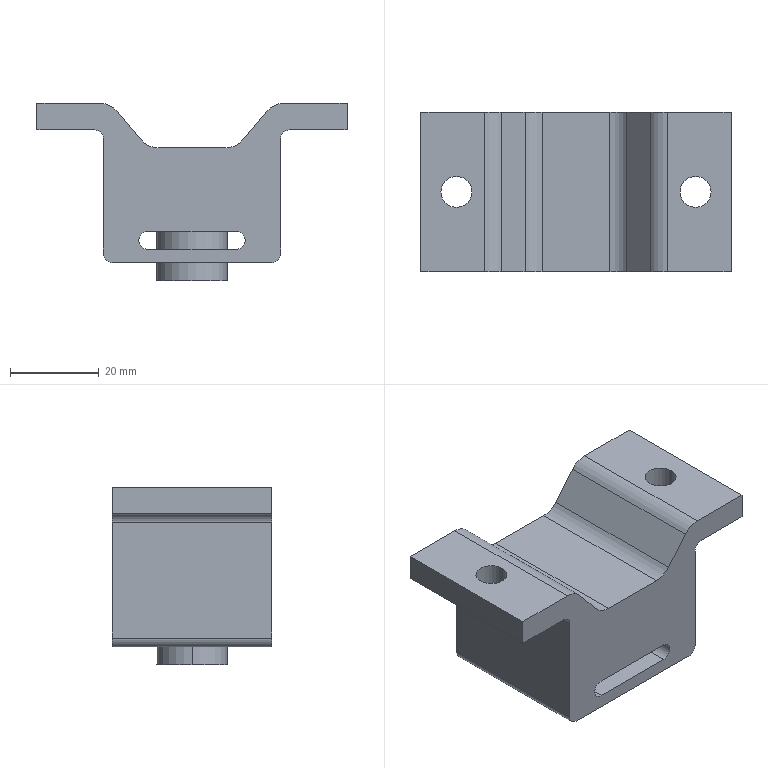Part | SolidWorks | features Fillet 3, ICE 3, Extrusion 1, HoleWzd 1 | 1 solid | 40 faces | box 70 x 36 x 40.002 mm | volume 44732 mm3 | cylinder 20 | plane 18 | cone 2 | commonest cylinder face diameters 4 x6 7 x4 10 x4 6.8 x2 16 x2 20 x2
STEP:
#1=CARTESIAN_POINT('',(3.4,18.,1.993));
#2=VERTEX_POINT('',#1);
#3=CARTESIAN_POINT('',(-3.4,18.,1.993));
#4=VERTEX_POINT('',#3);
#5=CARTESIAN_POINT('',(0.,18.,1.993));
#6=DIRECTION('',(0.,0.,-1.));
#7=DIRECTION('',(-1.,0.,0.));
#8=AXIS2_PLACEMENT_3D('',#5,#6,#7);
#9=CIRCLE('',#8,3.4);
#10=EDGE_CURVE('',#2,#4,#9,.T.);
#11=ORIENTED_EDGE('',*,*,#10,.F.);
#12=CARTESIAN_POINT('',(3.4,18.,-20.257));
#13=VERTEX_POINT('',#12);
#14=CARTESIAN_POINT('',(3.4,18.,-20.257));
#15=DIRECTION('',(0.,0.,-1.));
#16=VECTOR('',#15,1000.);
#17=LINE('',#14,#16);
#18=EDGE_CURVE('',#2,#13,#17,.T.);
#19=ORIENTED_EDGE('',*,*,#18,.T.);
#20=CARTESIAN_POINT('',(-3.4,18.,-20.257));
#21=VERTEX_POINT('',#20);
#22=CARTESIAN_POINT('',(0.,18.,-20.257));
#23=DIRECTION('',(0.,0.,-1.));
#24=DIRECTION('',(-1.,0.,0.));
#25=AXIS2_PLACEMENT_3D('',#22,#23,#24);
#26=CIRCLE('',#25,3.4);
#27=EDGE_CURVE('',#13,#21,#26,.T.);
#28=ORIENTED_EDGE('',*,*,#27,.T.);
#29=CARTESIAN_POINT('',(-3.4,18.,-20.257));
#30=DIRECTION('',(0.,0.,-1.));
#31=VECTOR('',#30,1000.);
#32=LINE('',#29,#31);
#33=EDGE_CURVE('',#4,#21,#32,.T.);
#34=ORIENTED_EDGE('',*,*,#33,.F.);
#35=EDGE_LOOP('',(#11,#19,#28,#34));
#36=FACE_OUTER_BOUND('',#35,.T.);
#37=CARTESIAN_POINT('',(0.,18.,-20.257));
#38=DIRECTION('',(0.,0.,-1.));
#39=DIRECTION('',(-1.,0.,0.));
#40=AXIS2_PLACEMENT_3D('',#37,#38,#39);
#41=CYLINDRICAL_SURFACE('',#40,3.4);
#42=ADVANCED_FACE('',(#36),#41,.F.);
#43=CARTESIAN_POINT('',(0.,18.,4.035));
#44=VERTEX_POINT('',#43);
#45=CARTESIAN_POINT('',(-3.4,18.,1.993));
#46=DIRECTION('',(-0.8572,0.,-0.515));
#47=VECTOR('',#46,1000.);
#48=LINE('',#45,#47);
#49=EDGE_CURVE('',#44,#4,#48,.T.);
#50=ORIENTED_EDGE('',*,*,#49,.F.);
#51=CARTESIAN_POINT('',(3.4,18.,1.993));
#52=DIRECTION('',(0.8572,0.,-0.515));
#53=VECTOR('',#52,1000.);
#54=LINE('',#51,#53);
#55=EDGE_CURVE('',#44,#2,#54,.T.);
#56=ORIENTED_EDGE('',*,*,#55,.T.);
#57=ORIENTED_EDGE('',*,*,#10,.T.);
#58=EDGE_LOOP('',(#50,#56,#57));
#59=FACE_OUTER_BOUND('',#58,.T.);
#60=CARTESIAN_POINT('',(0.,18.,1.993));
#61=DIRECTION('',(0.,0.,-1.));
#62=DIRECTION('',(-1.,0.,0.));
#63=AXIS2_PLACEMENT_3D('',#60,#61,#62);
#64=CONICAL_SURFACE('',#63,3.4,1.03);
#65=ADVANCED_FACE('',(#59),#64,.F.);
#66=CARTESIAN_POINT('',(-8.,18.,-20.257));
#67=VERTEX_POINT('',#66);
#68=CARTESIAN_POINT('',(8.,18.,-20.257));
#69=VERTEX_POINT('',#68);
#70=CARTESIAN_POINT('',(0.,18.,-20.257));
#71=DIRECTION('',(0.,0.,-1.));
#72=DIRECTION('',(-1.,0.,0.));
#73=AXIS2_PLACEMENT_3D('',#70,#71,#72);
#74=CIRCLE('',#73,8.);
#75=EDGE_CURVE('',#67,#69,#74,.T.);
#76=ORIENTED_EDGE('',*,*,#75,.F.);
#77=CARTESIAN_POINT('',(-8.,18.,-9.167));
#78=VERTEX_POINT('',#77);
#79=CARTESIAN_POINT('',(-8.,18.,-20.257));
#80=DIRECTION('',(0.,0.,1.));
#81=VECTOR('',#80,1000.);
#82=LINE('',#79,#81);
#83=EDGE_CURVE('',#67,#78,#82,.T.);
#84=ORIENTED_EDGE('',*,*,#83,.T.);
#85=CARTESIAN_POINT('',(8.,18.,-9.167));
#86=VERTEX_POINT('',#85);
#87=CARTESIAN_POINT('',(0.,18.,-9.167));
#88=DIRECTION('',(0.,0.,-1.));
#89=DIRECTION('',(-1.,0.,0.));
#90=AXIS2_PLACEMENT_3D('',#87,#88,#89);
#91=CIRCLE('',#90,8.);
#92=EDGE_CURVE('',#78,#86,#91,.T.);
#93=ORIENTED_EDGE('',*,*,#92,.T.);
#94=CARTESIAN_POINT('',(8.,18.,-20.257));
#95=DIRECTION('',(0.,0.,1.));
#96=VECTOR('',#95,1000.);
#97=LINE('',#94,#96);
#98=EDGE_CURVE('',#69,#86,#97,.T.);
#99=ORIENTED_EDGE('',*,*,#98,.F.);
#100=EDGE_LOOP('',(#76,#84,#93,#99));
#101=FACE_OUTER_BOUND('',#100,.T.);
#102=CARTESIAN_POINT('',(0.,18.,-20.257));
#103=DIRECTION('',(0.,0.,1.));
#104=DIRECTION('',(1.,0.,0.));
#105=AXIS2_PLACEMENT_3D('',#102,#103,#104);
#106=CYLINDRICAL_SURFACE('',#105,8.);
#107=ADVANCED_FACE('',(#101),#106,.T.);
#108=CARTESIAN_POINT('',(-10.,18.,-13.167));
#109=VERTEX_POINT('',#108);
#110=CARTESIAN_POINT('',(10.,18.,-13.167));
#111=VERTEX_POINT('',#110);
#112=CARTESIAN_POINT('',(0.,18.,-13.167));
#113=DIRECTION('',(0.,0.,1.));
#114=DIRECTION('',(1.,0.,0.));
#115=AXIS2_PLACEMENT_3D('',#112,#113,#114);
#116=CIRCLE('',#115,10.);
#117=EDGE_CURVE('',#109,#111,#116,.T.);
#118=ORIENTED_EDGE('',*,*,#117,.T.);
#119=CARTESIAN_POINT('',(10.,18.,-16.255));
#120=VERTEX_POINT('',#119);
#121=CARTESIAN_POINT('',(10.,18.,-10.255));
#122=DIRECTION('',(0.,0.,-1.));
#123=VECTOR('',#122,1000.);
#124=LINE('',#121,#123);
#125=EDGE_CURVE('',#111,#120,#124,.T.);
#126=ORIENTED_EDGE('',*,*,#125,.T.);
#127=CARTESIAN_POINT('',(-10.,18.,-16.255));
#128=VERTEX_POINT('',#127);
#129=CARTESIAN_POINT('',(0.,18.,-16.255));
#130=DIRECTION('',(0.,0.,-1.));
#131=DIRECTION('',(-1.,0.,0.));
#132=AXIS2_PLACEMENT_3D('',#129,#130,#131);
#133=CIRCLE('',#132,10.);
#134=EDGE_CURVE('',#120,#128,#133,.T.);
#135=ORIENTED_EDGE('',*,*,#134,.T.);
#136=CARTESIAN_POINT('',(-10.,18.,-10.255));
#137=DIRECTION('',(0.,0.,-1.));
#138=VECTOR('',#137,1000.);
#139=LINE('',#136,#138);
#140=EDGE_CURVE('',#109,#128,#139,.T.);
#141=ORIENTED_EDGE('',*,*,#140,.F.);
#142=EDGE_LOOP('',(#118,#126,#135,#141));
#143=FACE_OUTER_BOUND('',#142,.T.);
#144=CARTESIAN_POINT('',(0.,18.,-10.255));
#145=DIRECTION('',(0.,0.,-1.));
#146=DIRECTION('',(-1.,0.,0.));
#147=AXIS2_PLACEMENT_3D('',#144,#145,#146);
#148=CYLINDRICAL_SURFACE('',#147,10.);
#149=ADVANCED_FACE('',(#143),#148,.F.);
#150=CARTESIAN_POINT('',(-23.5,18.,19.745));
#151=VERTEX_POINT('',#150);
#152=CARTESIAN_POINT('',(-30.5,18.,19.745));
#153=VERTEX_POINT('',#152);
#154=CARTESIAN_POINT('',(-27.,18.,19.745));
#155=DIRECTION('',(0.,0.,-1.));
#156=DIRECTION('',(-1.,0.,0.));
#157=AXIS2_PLACEMENT_3D('',#154,#155,#156);
#158=CIRCLE('',#157,3.5);
#159=EDGE_CURVE('',#151,#153,#158,.T.);
#160=ORIENTED_EDGE('',*,*,#159,.F.);
#161=CARTESIAN_POINT('',(-23.5,18.,13.745));
#162=VERTEX_POINT('',#161);
#163=CARTESIAN_POINT('',(-23.5,18.,19.745));
#164=DIRECTION('',(0.,0.,-1.));
#165=VECTOR('',#164,1000.);
#166=LINE('',#163,#165);
#167=EDGE_CURVE('',#151,#162,#166,.T.);
#168=ORIENTED_EDGE('',*,*,#167,.T.);
#169=CARTESIAN_POINT('',(-30.5,18.,13.745));
#170=VERTEX_POINT('',#169);
#171=CARTESIAN_POINT('',(-27.,18.,13.745));
#172=DIRECTION('',(0.,0.,-1.));
#173=DIRECTION('',(-1.,0.,0.));
#174=AXIS2_PLACEMENT_3D('',#171,#172,#173);
#175=CIRCLE('',#174,3.5);
#176=EDGE_CURVE('',#162,#170,#175,.T.);
#177=ORIENTED_EDGE('',*,*,#176,.T.);
#178=CARTESIAN_POINT('',(-30.5,18.,19.745));
#179=DIRECTION('',(0.,0.,-1.));
#180=VECTOR('',#179,1000.);
#181=LINE('',#178,#180);
#182=EDGE_CURVE('',#153,#170,#181,.T.);
#183=ORIENTED_EDGE('',*,*,#182,.F.);
#184=EDGE_LOOP('',(#160,#168,#177,#183));
#185=FACE_OUTER_BOUND('',#184,.T.);
#186=CARTESIAN_POINT('',(-27.,18.,19.745));
#187=DIRECTION('',(0.,0.,-1.));
#188=DIRECTION('',(-1.,0.,0.));
#189=AXIS2_PLACEMENT_3D('',#186,#187,#188);
#190=CYLINDRICAL_SURFACE('',#189,3.5);
#191=ADVANCED_FACE('',(#185),#190,.F.);
#192=CARTESIAN_POINT('',(30.5,18.,19.745));
#193=VERTEX_POINT('',#192);
#194=CARTESIAN_POINT('',(23.5,18.,19.745));
#195=VERTEX_POINT('',#194);
#196=CARTESIAN_POINT('',(27.,18.,19.745));
#197=DIRECTION('',(0.,0.,-1.));
#198=DIRECTION('',(-1.,0.,0.));
#199=AXIS2_PLACEMENT_3D('',#196,#197,#198);
#200=CIRCLE('',#199,3.5);
#201=EDGE_CURVE('',#193,#195,#200,.T.);
#202=ORIENTED_EDGE('',*,*,#201,.F.);
#203=CARTESIAN_POINT('',(30.5,18.,13.745));
#204=VERTEX_POINT('',#203);
#205=CARTESIAN_POINT('',(30.5,18.,19.745));
#206=DIRECTION('',(0.,0.,-1.));
#207=VECTOR('',#206,1000.);
#208=LINE('',#205,#207);
#209=EDGE_CURVE('',#193,#204,#208,.T.);
#210=ORIENTED_EDGE('',*,*,#209,.T.);
#211=CARTESIAN_POINT('',(23.5,18.,13.745));
#212=VERTEX_POINT('',#211);
#213=CARTESIAN_POINT('',(27.,18.,13.745));
#214=DIRECTION('',(0.,0.,-1.));
#215=DIRECTION('',(-1.,0.,0.));
#216=AXIS2_PLACEMENT_3D('',#213,#214,#215);
#217=CIRCLE('',#216,3.5);
#218=EDGE_CURVE('',#204,#212,#217,.T.);
#219=ORIENTED_EDGE('',*,*,#218,.T.);
#220=CARTESIAN_POINT('',(23.5,18.,19.745));
#221=DIRECTION('',(0.,0.,-1.));
#222=VECTOR('',#221,1000.);
#223=LINE('',#220,#222);
#224=EDGE_CURVE('',#195,#212,#223,.T.);
#225=ORIENTED_EDGE('',*,*,#224,.F.);
#226=EDGE_LOOP('',(#202,#210,#219,#225));
#227=FACE_OUTER_BOUND('',#226,.T.);
#228=CARTESIAN_POINT('',(27.,18.,19.745));
#229=DIRECTION('',(0.,0.,-1.));
#230=DIRECTION('',(-1.,0.,0.));
#231=AXIS2_PLACEMENT_3D('',#228,#229,#230);
#232=CYLINDRICAL_SURFACE('',#231,3.5);
#233=ADVANCED_FACE('',(#227),#232,.F.);
#234=CARTESIAN_POINT('',(0.,18.,-13.167));
#235=DIRECTION('',(0.,0.,1.));
#236=DIRECTION('',(1.,0.,0.));
#237=AXIS2_PLACEMENT_3D('',#234,#235,#236);
#238=CIRCLE('',#237,10.);
#239=EDGE_CURVE('',#111,#109,#238,.T.);
#240=ORIENTED_EDGE('',*,*,#239,.F.);
#241=CARTESIAN_POINT('',(10.,36.,-13.167));
#242=VERTEX_POINT('',#241);
#243=CARTESIAN_POINT('',(10.,36.,-13.167));
#244=DIRECTION('',(0.,-1.,0.));
#245=VECTOR('',#244,1000.);
#246=LINE('',#243,#245);
#247=EDGE_CURVE('',#242,#111,#246,.T.);
#248=ORIENTED_EDGE('',*,*,#247,.F.);
#249=CARTESIAN_POINT('',(-10.,36.,-13.167));
#250=VERTEX_POINT('',#249);
#251=CARTESIAN_POINT('',(-10.,36.,-13.167));
#252=DIRECTION('',(-1.,0.,0.));
#253=VECTOR('',#252,1000.);
#254=LINE('',#251,#253);
#255=EDGE_CURVE('',#242,#250,#254,.T.);
#256=ORIENTED_EDGE('',*,*,#255,.T.);
#257=CARTESIAN_POINT('',(-10.,36.,-13.167));
#258=DIRECTION('',(0.,-1.,0.));
#259=VECTOR('',#258,1000.);
#260=LINE('',#257,#259);
#261=EDGE_CURVE('',#250,#109,#260,.T.);
#262=ORIENTED_EDGE('',*,*,#261,.T.);
#263=EDGE_LOOP('',(#240,#248,#256,#262));
#264=FACE_OUTER_BOUND('',#263,.T.);
#265=CARTESIAN_POINT('',(-10.,36.,-13.167));
#266=DIRECTION('',(0.,0.,1.));
#267=DIRECTION('',(1.,0.,0.));
#268=AXIS2_PLACEMENT_3D('',#265,#266,#267);
#269=PLANE('',#268);
#270=ADVANCED_FACE('',(#264),#269,.T.);
#271=CARTESIAN_POINT('',(18.,36.,-16.255));
#272=VERTEX_POINT('',#271);
#273=CARTESIAN_POINT('',(-18.,36.,-16.255));
#274=VERTEX_POINT('',#273);
#275=CARTESIAN_POINT('',(-20.,36.,-16.255));
#276=DIRECTION('',(-1.,0.,0.));
#277=VECTOR('',#276,1000.);
#278=LINE('',#275,#277);
#279=EDGE_CURVE('',#272,#274,#278,.T.);
#280=ORIENTED_EDGE('',*,*,#279,.T.);
#281=CARTESIAN_POINT('',(-20.,36.,-14.255));
#282=VERTEX_POINT('',#281);
#283=CARTESIAN_POINT('',(-18.,36.,-14.255));
#284=DIRECTION('',(0.,1.,0.));
#285=DIRECTION('',(0.,0.,-1.));
#286=AXIS2_PLACEMENT_3D('',#283,#284,#285);
#287=CIRCLE('',#286,2.);
#288=EDGE_CURVE('',#274,#282,#287,.T.);
#289=ORIENTED_EDGE('',*,*,#288,.T.);
#290=CARTESIAN_POINT('',(-20.,36.,11.745));
#291=VERTEX_POINT('',#290);
#292=CARTESIAN_POINT('',(-20.,36.,13.745));
#293=DIRECTION('',(0.,0.,1.));
#294=VECTOR('',#293,1000.);
#295=LINE('',#292,#294);
#296=EDGE_CURVE('',#282,#291,#295,.T.);
#297=ORIENTED_EDGE('',*,*,#296,.T.);
#298=CARTESIAN_POINT('',(-22.,36.,13.745));
#299=VERTEX_POINT('',#298);
#300=CARTESIAN_POINT('',(-22.,36.,11.745));
#301=DIRECTION('',(0.,-1.,0.));
#302=DIRECTION('',(0.,0.,-1.));
#303=AXIS2_PLACEMENT_3D('',#300,#301,#302);
#304=CIRCLE('',#303,2.);
#305=EDGE_CURVE('',#291,#299,#304,.T.);
#306=ORIENTED_EDGE('',*,*,#305,.T.);
#307=CARTESIAN_POINT('',(-35.,36.,13.745));
#308=VERTEX_POINT('',#307);
#309=CARTESIAN_POINT('',(-35.,36.,13.745));
#310=DIRECTION('',(-1.,0.,0.));
#311=VECTOR('',#310,1000.);
#312=LINE('',#309,#311);
#313=EDGE_CURVE('',#299,#308,#312,.T.);
#314=ORIENTED_EDGE('',*,*,#313,.T.);
#315=CARTESIAN_POINT('',(-35.,36.,19.745));
#316=VERTEX_POINT('',#315);
#317=CARTESIAN_POINT('',(-35.,36.,19.745));
#318=DIRECTION('',(0.,0.,1.));
#319=VECTOR('',#318,1000.);
#320=LINE('',#317,#319);
#321=EDGE_CURVE('',#308,#316,#320,.T.);
#322=ORIENTED_EDGE('',*,*,#321,.T.);
#323=CARTESIAN_POINT('',(-20.723,36.,19.745));
#324=VERTEX_POINT('',#323);
#325=CARTESIAN_POINT('',(-35.,36.,19.745));
#326=DIRECTION('',(1.,0.,0.));
#327=VECTOR('',#326,1000.);
#328=LINE('',#325,#327);
#329=EDGE_CURVE('',#316,#324,#328,.T.);
#330=ORIENTED_EDGE('',*,*,#329,.T.);
#331=CARTESIAN_POINT('',(-16.892,36.,17.959));
#332=VERTEX_POINT('',#331);
#333=CARTESIAN_POINT('',(-20.723,36.,14.745));
#334=DIRECTION('',(0.,1.,0.));
#335=DIRECTION('',(0.,0.,-1.));
#336=AXIS2_PLACEMENT_3D('',#333,#334,#335);
#337=CIRCLE('',#336,5.);
#338=EDGE_CURVE('',#324,#332,#337,.T.);
#339=ORIENTED_EDGE('',*,*,#338,.T.);
#340=CARTESIAN_POINT('',(-11.499,36.,11.531));
#341=VERTEX_POINT('',#340);
#342=CARTESIAN_POINT('',(-18.391,36.,19.745));
#343=DIRECTION('',(0.6428,0.,-0.766));
#344=VECTOR('',#343,1000.);
#345=LINE('',#342,#344);
#346=EDGE_CURVE('',#332,#341,#345,.T.);
#347=ORIENTED_EDGE('',*,*,#346,.T.);
#348=CARTESIAN_POINT('',(-7.668,36.,9.745));
#349=VERTEX_POINT('',#348);
#350=CARTESIAN_POINT('',(-7.668,36.,14.745));
#351=DIRECTION('',(0.,-1.,0.));
#352=DIRECTION('',(0.,0.,-1.));
#353=AXIS2_PLACEMENT_3D('',#350,#351,#352);
#354=CIRCLE('',#353,5.);
#355=EDGE_CURVE('',#341,#349,#354,.T.);
#356=ORIENTED_EDGE('',*,*,#355,.T.);
#357=CARTESIAN_POINT('',(7.668,36.,9.745));
#358=VERTEX_POINT('',#357);
#359=CARTESIAN_POINT('',(-10.,36.,9.745));
#360=DIRECTION('',(1.,0.,0.));
#361=VECTOR('',#360,1000.);
#362=LINE('',#359,#361);
#363=EDGE_CURVE('',#349,#358,#362,.T.);
#364=ORIENTED_EDGE('',*,*,#363,.T.);
#365=CARTESIAN_POINT('',(11.499,36.,11.531));
#366=VERTEX_POINT('',#365);
#367=CARTESIAN_POINT('',(7.668,36.,14.745));
#368=DIRECTION('',(0.,-1.,0.));
#369=DIRECTION('',(0.,0.,-1.));
#370=AXIS2_PLACEMENT_3D('',#367,#368,#369);
#371=CIRCLE('',#370,5.);
#372=EDGE_CURVE('',#358,#366,#371,.T.);
#373=ORIENTED_EDGE('',*,*,#372,.T.);
#374=CARTESIAN_POINT('',(16.892,36.,17.959));
#375=VERTEX_POINT('',#374);
#376=CARTESIAN_POINT('',(10.,36.,9.745));
#377=DIRECTION('',(0.6428,0.,0.766));
#378=VECTOR('',#377,1000.);
#379=LINE('',#376,#378);
#380=EDGE_CURVE('',#366,#375,#379,.T.);
#381=ORIENTED_EDGE('',*,*,#380,.T.);
#382=CARTESIAN_POINT('',(20.723,36.,19.745));
#383=VERTEX_POINT('',#382);
#384=CARTESIAN_POINT('',(20.723,36.,14.745));
#385=DIRECTION('',(0.,1.,0.));
#386=DIRECTION('',(0.,0.,-1.));
#387=AXIS2_PLACEMENT_3D('',#384,#385,#386);
#388=CIRCLE('',#387,5.);
#389=EDGE_CURVE('',#375,#383,#388,.T.);
#390=ORIENTED_EDGE('',*,*,#389,.T.);
#391=CARTESIAN_POINT('',(35.,36.,19.745));
#392=VERTEX_POINT('',#391);
#393=CARTESIAN_POINT('',(18.391,36.,19.745));
#394=DIRECTION('',(1.,0.,0.));
#395=VECTOR('',#394,1000.);
#396=LINE('',#393,#395);
#397=EDGE_CURVE('',#383,#392,#396,.T.);
#398=ORIENTED_EDGE('',*,*,#397,.T.);
#399=CARTESIAN_POINT('',(35.,36.,13.745));
#400=VERTEX_POINT('',#399);
#401=CARTESIAN_POINT('',(35.,36.,19.745));
#402=DIRECTION('',(0.,0.,-1.));
#403=VECTOR('',#402,1000.);
#404=LINE('',#401,#403);
#405=EDGE_CURVE('',#392,#400,#404,.T.);
#406=ORIENTED_EDGE('',*,*,#405,.T.);
#407=CARTESIAN_POINT('',(22.,36.,13.745));
#408=VERTEX_POINT('',#407);
#409=CARTESIAN_POINT('',(20.,36.,13.745));
#410=DIRECTION('',(-1.,0.,0.));
#411=VECTOR('',#410,1000.);
#412=LINE('',#409,#411);
#413=EDGE_CURVE('',#400,#408,#412,.T.);
#414=ORIENTED_EDGE('',*,*,#413,.T.);
#415=CARTESIAN_POINT('',(20.,36.,11.745));
#416=VERTEX_POINT('',#415);
#417=CARTESIAN_POINT('',(22.,36.,11.745));
#418=DIRECTION('',(0.,-1.,0.));
#419=DIRECTION('',(0.,0.,-1.));
#420=AXIS2_PLACEMENT_3D('',#417,#418,#419);
#421=CIRCLE('',#420,2.);
#422=EDGE_CURVE('',#408,#416,#421,.T.);
#423=ORIENTED_EDGE('',*,*,#422,.T.);
#424=CARTESIAN_POINT('',(20.,36.,-14.255));
#425=VERTEX_POINT('',#424);
#426=CARTESIAN_POINT('',(20.,36.,13.745));
#427=DIRECTION('',(0.,0.,-1.));
#428=VECTOR('',#427,1000.);
#429=LINE('',#426,#428);
#430=EDGE_CURVE('',#416,#425,#429,.T.);
#431=ORIENTED_EDGE('',*,*,#430,.T.);
#432=CARTESIAN_POINT('',(18.,36.,-14.255));
#433=DIRECTION('',(0.,1.,0.));
#434=DIRECTION('',(0.,0.,-1.));
#435=AXIS2_PLACEMENT_3D('',#432,#433,#434);
#436=CIRCLE('',#435,2.);
#437=EDGE_CURVE('',#425,#272,#436,.T.);
#438=ORIENTED_EDGE('',*,*,#437,.T.);
#439=EDGE_LOOP('',(#280,#289,#297,#306,#314,#322,#330,#339,#347,#356,#364,#373,#381,#390,#398,#406,#414,#423,#431,#438));
#440=FACE_OUTER_BOUND('',#439,.T.);
#441=CARTESIAN_POINT('',(-10.,36.,-9.167));
#442=VERTEX_POINT('',#441);
#443=CARTESIAN_POINT('',(-10.,36.,-11.167));
#444=DIRECTION('',(0.,1.,0.));
#445=DIRECTION('',(0.,0.,1.));
#446=AXIS2_PLACEMENT_3D('',#443,#444,#445);
#447=CIRCLE('',#446,2.);
#448=EDGE_CURVE('',#250,#442,#447,.T.);
#449=ORIENTED_EDGE('',*,*,#448,.F.);
#450=ORIENTED_EDGE('',*,*,#255,.F.);
#451=CARTESIAN_POINT('',(10.,36.,-9.167));
#452=VERTEX_POINT('',#451);
#453=CARTESIAN_POINT('',(10.,36.,-11.167));
#454=DIRECTION('',(0.,1.,0.));
#455=DIRECTION('',(0.,0.,1.));
#456=AXIS2_PLACEMENT_3D('',#453,#454,#455);
#457=CIRCLE('',#456,2.);
#458=EDGE_CURVE('',#452,#242,#457,.T.);
#459=ORIENTED_EDGE('',*,*,#458,.F.);
#460=CARTESIAN_POINT('',(-10.,36.,-9.167));
#461=DIRECTION('',(1.,0.,0.));
#462=VECTOR('',#461,1000.);
#463=LINE('',#460,#462);
#464=EDGE_CURVE('',#442,#452,#463,.T.);
#465=ORIENTED_EDGE('',*,*,#464,.F.);
#466=EDGE_LOOP('',(#449,#450,#459,#465));
#467=FACE_BOUND('',#466,.T.);
#468=CARTESIAN_POINT('',(0.,36.,0.));
#469=DIRECTION('',(0.,-1.,0.));
#470=DIRECTION('',(0.,0.,-1.));
#471=AXIS2_PLACEMENT_3D('',#468,#469,#470);
#472=PLANE('',#471);
#473=ADVANCED_FACE('',(#440,#467),#472,.F.);
#474=CARTESIAN_POINT('',(-20.,0.,-14.255));
#475=VERTEX_POINT('',#474);
#476=CARTESIAN_POINT('',(-20.,0.,11.745));
#477=VERTEX_POINT('',#476);
#478=CARTESIAN_POINT('',(-20.,0.,13.745));
#479=DIRECTION('',(0.,0.,1.));
#480=VECTOR('',#479,1000.);
#481=LINE('',#478,#480);
#482=EDGE_CURVE('',#475,#477,#481,.T.);
#483=ORIENTED_EDGE('',*,*,#482,.F.);
#484=CARTESIAN_POINT('',(-18.,0.,-16.255));
#485=VERTEX_POINT('',#484);
#486=CARTESIAN_POINT('',(-18.,0.,-14.255));
#487=DIRECTION('',(0.,-1.,0.));
#488=DIRECTION('',(0.,0.,-1.));
#489=AXIS2_PLACEMENT_3D('',#486,#487,#488);
#490=CIRCLE('',#489,2.);
#491=EDGE_CURVE('',#475,#485,#490,.T.);
#492=ORIENTED_EDGE('',*,*,#491,.T.);
#493=CARTESIAN_POINT('',(18.,0.,-16.255));
#494=VERTEX_POINT('',#493);
#495=CARTESIAN_POINT('',(-20.,0.,-16.255));
#496=DIRECTION('',(-1.,0.,0.));
#497=VECTOR('',#496,1000.);
#498=LINE('',#495,#497);
#499=EDGE_CURVE('',#494,#485,#498,.T.);
#500=ORIENTED_EDGE('',*,*,#499,.F.);
#501=CARTESIAN_POINT('',(20.,0.,-14.255));
#502=VERTEX_POINT('',#501);
#503=CARTESIAN_POINT('',(18.,0.,-14.255));
#504=DIRECTION('',(0.,-1.,0.));
#505=DIRECTION('',(0.,0.,-1.));
#506=AXIS2_PLACEMENT_3D('',#503,#504,#505);
#507=CIRCLE('',#506,2.);
#508=EDGE_CURVE('',#494,#502,#507,.T.);
#509=ORIENTED_EDGE('',*,*,#508,.T.);
#510=CARTESIAN_POINT('',(20.,0.,11.745));
#511=VERTEX_POINT('',#510);
#512=CARTESIAN_POINT('',(20.,0.,13.745));
#513=DIRECTION('',(0.,0.,-1.));
#514=VECTOR('',#513,1000.);
#515=LINE('',#512,#514);
#516=EDGE_CURVE('',#511,#502,#515,.T.);
#517=ORIENTED_EDGE('',*,*,#516,.F.);
#518=CARTESIAN_POINT('',(22.,0.,13.745));
#519=VERTEX_POINT('',#518);
#520=CARTESIAN_POINT('',(22.,0.,11.745));
#521=DIRECTION('',(0.,1.,0.));
#522=DIRECTION('',(0.,0.,-1.));
#523=AXIS2_PLACEMENT_3D('',#520,#521,#522);
#524=CIRCLE('',#523,2.);
#525=EDGE_CURVE('',#511,#519,#524,.T.);
#526=ORIENTED_EDGE('',*,*,#525,.T.);
#527=CARTESIAN_POINT('',(35.,0.,13.745));
#528=VERTEX_POINT('',#527);
#529=CARTESIAN_POINT('',(20.,0.,13.745));
#530=DIRECTION('',(-1.,0.,0.));
#531=VECTOR('',#530,1000.);
#532=LINE('',#529,#531);
#533=EDGE_CURVE('',#528,#519,#532,.T.);
#534=ORIENTED_EDGE('',*,*,#533,.F.);
#535=CARTESIAN_POINT('',(35.,0.,19.745));
#536=VERTEX_POINT('',#535);
#537=CARTESIAN_POINT('',(35.,0.,19.745));
#538=DIRECTION('',(0.,0.,-1.));
#539=VECTOR('',#538,1000.);
#540=LINE('',#537,#539);
#541=EDGE_CURVE('',#536,#528,#540,.T.);
#542=ORIENTED_EDGE('',*,*,#541,.F.);
#543=CARTESIAN_POINT('',(20.723,0.,19.745));
#544=VERTEX_POINT('',#543);
#545=CARTESIAN_POINT('',(18.391,0.,19.745));
#546=DIRECTION('',(1.,0.,0.));
#547=VECTOR('',#546,1000.);
#548=LINE('',#545,#547);
#549=EDGE_CURVE('',#544,#536,#548,.T.);
#550=ORIENTED_EDGE('',*,*,#549,.F.);
#551=CARTESIAN_POINT('',(16.892,0.,17.959));
#552=VERTEX_POINT('',#551);
#553=CARTESIAN_POINT('',(20.723,0.,14.745));
#554=DIRECTION('',(0.,-1.,0.));
#555=DIRECTION('',(0.,0.,-1.));
#556=AXIS2_PLACEMENT_3D('',#553,#554,#555);
#557=CIRCLE('',#556,5.);
#558=EDGE_CURVE('',#544,#552,#557,.T.);
#559=ORIENTED_EDGE('',*,*,#558,.T.);
#560=CARTESIAN_POINT('',(11.499,0.,11.531));
#561=VERTEX_POINT('',#560);
#562=CARTESIAN_POINT('',(10.,0.,9.745));
#563=DIRECTION('',(0.6428,0.,0.766));
#564=VECTOR('',#563,1000.);
#565=LINE('',#562,#564);
#566=EDGE_CURVE('',#561,#552,#565,.T.);
#567=ORIENTED_EDGE('',*,*,#566,.F.);
#568=CARTESIAN_POINT('',(7.668,0.,9.745));
#569=VERTEX_POINT('',#568);
#570=CARTESIAN_POINT('',(7.668,0.,14.745));
#571=DIRECTION('',(0.,1.,0.));
#572=DIRECTION('',(0.,0.,-1.));
#573=AXIS2_PLACEMENT_3D('',#570,#571,#572);
#574=CIRCLE('',#573,5.);
#575=EDGE_CURVE('',#561,#569,#574,.T.);
#576=ORIENTED_EDGE('',*,*,#575,.T.);
#577=CARTESIAN_POINT('',(-7.668,0.,9.745));
#578=VERTEX_POINT('',#577);
#579=CARTESIAN_POINT('',(-10.,0.,9.745));
#580=DIRECTION('',(1.,0.,0.));
#581=VECTOR('',#580,1000.);
#582=LINE('',#579,#581);
#583=EDGE_CURVE('',#578,#569,#582,.T.);
#584=ORIENTED_EDGE('',*,*,#583,.F.);
#585=CARTESIAN_POINT('',(-11.499,0.,11.531));
#586=VERTEX_POINT('',#585);
#587=CARTESIAN_POINT('',(-7.668,0.,14.745));
#588=DIRECTION('',(0.,1.,0.));
#589=DIRECTION('',(0.,0.,-1.));
#590=AXIS2_PLACEMENT_3D('',#587,#588,#589);
#591=CIRCLE('',#590,5.);
#592=EDGE_CURVE('',#578,#586,#591,.T.);
#593=ORIENTED_EDGE('',*,*,#592,.T.);
#594=CARTESIAN_POINT('',(-16.892,0.,17.959));
#595=VERTEX_POINT('',#594);
#596=CARTESIAN_POINT('',(-18.391,0.,19.745));
#597=DIRECTION('',(0.6428,0.,-0.766));
#598=VECTOR('',#597,1000.);
#599=LINE('',#596,#598);
#600=EDGE_CURVE('',#595,#586,#599,.T.);
#601=ORIENTED_EDGE('',*,*,#600,.F.);
#602=CARTESIAN_POINT('',(-20.723,0.,19.745));
#603=VERTEX_POINT('',#602);
#604=CARTESIAN_POINT('',(-20.723,0.,14.745));
#605=DIRECTION('',(0.,-1.,0.));
#606=DIRECTION('',(0.,0.,-1.));
#607=AXIS2_PLACEMENT_3D('',#604,#605,#606);
#608=CIRCLE('',#607,5.);
#609=EDGE_CURVE('',#595,#603,#608,.T.);
#610=ORIENTED_EDGE('',*,*,#609,.T.);
#611=CARTESIAN_POINT('',(-35.,0.,19.745));
#612=VERTEX_POINT('',#611);
#613=CARTESIAN_POINT('',(-35.,0.,19.745));
#614=DIRECTION('',(1.,0.,0.));
#615=VECTOR('',#614,1000.);
#616=LINE('',#613,#615);
#617=EDGE_CURVE('',#612,#603,#616,.T.);
#618=ORIENTED_EDGE('',*,*,#617,.F.);
#619=CARTESIAN_POINT('',(-35.,0.,13.745));
#620=VERTEX_POINT('',#619);
#621=CARTESIAN_POINT('',(-35.,0.,19.745));
#622=DIRECTION('',(0.,0.,1.));
#623=VECTOR('',#622,1000.);
#624=LINE('',#621,#623);
#625=EDGE_CURVE('',#620,#612,#624,.T.);
#626=ORIENTED_EDGE('',*,*,#625,.F.);
#627=CARTESIAN_POINT('',(-22.,0.,13.745));
#628=VERTEX_POINT('',#627);
#629=CARTESIAN_POINT('',(-35.,0.,13.745));
#630=DIRECTION('',(-1.,0.,0.));
#631=VECTOR('',#630,1000.);
#632=LINE('',#629,#631);
#633=EDGE_CURVE('',#628,#620,#632,.T.);
#634=ORIENTED_EDGE('',*,*,#633,.F.);
#635=CARTESIAN_POINT('',(-22.,0.,11.745));
#636=DIRECTION('',(0.,1.,0.));
#637=DIRECTION('',(0.,0.,-1.));
#638=AXIS2_PLACEMENT_3D('',#635,#636,#637);
#639=CIRCLE('',#638,2.);
#640=EDGE_CURVE('',#628,#477,#639,.T.);
#641=ORIENTED_EDGE('',*,*,#640,.T.);
#642=EDGE_LOOP('',(#483,#492,#500,#509,#517,#526,#534,#542,#550,#559,#567,#576,#584,#593,#601,#610,#618,#626,#634,#641));
#643=FACE_OUTER_BOUND('',#642,.T.);
#644=CARTESIAN_POINT('',(10.,0.,-13.167));
#645=VERTEX_POINT('',#644);
#646=CARTESIAN_POINT('',(-10.,0.,-13.167));
#647=VERTEX_POINT('',#646);
#648=CARTESIAN_POINT('',(-10.,0.,-13.167));
#649=DIRECTION('',(-1.,0.,0.));
#650=VECTOR('',#649,1000.);
#651=LINE('',#648,#650);
#652=EDGE_CURVE('',#645,#647,#651,.T.);
#653=ORIENTED_EDGE('',*,*,#652,.T.);
#654=CARTESIAN_POINT('',(-10.,0.,-9.167));
#655=VERTEX_POINT('',#654);
#656=CARTESIAN_POINT('',(-10.,0.,-11.167));
#657=DIRECTION('',(0.,1.,0.));
#658=DIRECTION('',(0.,0.,1.));
#659=AXIS2_PLACEMENT_3D('',#656,#657,#658);
#660=CIRCLE('',#659,2.);
#661=EDGE_CURVE('',#647,#655,#660,.T.);
#662=ORIENTED_EDGE('',*,*,#661,.T.);
#663=CARTESIAN_POINT('',(10.,0.,-9.167));
#664=VERTEX_POINT('',#663);
#665=CARTESIAN_POINT('',(-10.,0.,-9.167));
#666=DIRECTION('',(1.,0.,0.));
#667=VECTOR('',#666,1000.);
#668=LINE('',#665,#667);
#669=EDGE_CURVE('',#655,#664,#668,.T.);
#670=ORIENTED_EDGE('',*,*,#669,.T.);
#671=CARTESIAN_POINT('',(10.,0.,-11.167));
#672=DIRECTION('',(0.,1.,0.));
#673=DIRECTION('',(0.,0.,1.));
#674=AXIS2_PLACEMENT_3D('',#671,#672,#673);
#675=CIRCLE('',#674,2.);
#676=EDGE_CURVE('',#664,#645,#675,.T.);
#677=ORIENTED_EDGE('',*,*,#676,.T.);
#678=EDGE_LOOP('',(#653,#662,#670,#677));
#679=FACE_BOUND('',#678,.T.);
#680=CARTESIAN_POINT('',(0.,0.,0.));
#681=DIRECTION('',(0.,-1.,0.));
#682=DIRECTION('',(0.,0.,-1.));
#683=AXIS2_PLACEMENT_3D('',#680,#681,#682);
#684=PLANE('',#683);
#685=ADVANCED_FACE('',(#643,#679),#684,.T.);
#686=ORIENTED_EDGE('',*,*,#516,.T.);
#687=CARTESIAN_POINT('',(20.,36.,-14.255));
#688=DIRECTION('',(0.,1.,0.));
#689=VECTOR('',#688,1000.);
#690=LINE('',#687,#689);
#691=EDGE_CURVE('',#502,#425,#690,.T.);
#692=ORIENTED_EDGE('',*,*,#691,.T.);
#693=ORIENTED_EDGE('',*,*,#430,.F.);
#694=CARTESIAN_POINT('',(20.,0.,11.745));
#695=DIRECTION('',(0.,-1.,0.));
#696=VECTOR('',#695,1000.);
#697=LINE('',#694,#696);
#698=EDGE_CURVE('',#416,#511,#697,.T.);
#699=ORIENTED_EDGE('',*,*,#698,.T.);
#700=EDGE_LOOP('',(#686,#692,#693,#699));
#701=FACE_OUTER_BOUND('',#700,.T.);
#702=CARTESIAN_POINT('',(20.,36.,13.745));
#703=DIRECTION('',(-1.,0.,0.));
#704=DIRECTION('',(0.,0.,1.));
#705=AXIS2_PLACEMENT_3D('',#702,#703,#704);
#706=PLANE('',#705);
#707=ADVANCED_FACE('',(#701),#706,.F.);
#708=CARTESIAN_POINT('',(0.,18.,-16.255));
#709=DIRECTION('',(0.,0.,-1.));
#710=DIRECTION('',(-1.,0.,0.));
#711=AXIS2_PLACEMENT_3D('',#708,#709,#710);
#712=CIRCLE('',#711,10.);
#713=EDGE_CURVE('',#128,#120,#712,.T.);
#714=ORIENTED_EDGE('',*,*,#713,.F.);
#715=ORIENTED_EDGE('',*,*,#134,.F.);
#716=EDGE_LOOP('',(#714,#715));
#717=FACE_BOUND('',#716,.T.);
#718=ORIENTED_EDGE('',*,*,#499,.T.);
#719=CARTESIAN_POINT('',(-18.,36.,-16.255));
#720=DIRECTION('',(0.,1.,0.));
#721=VECTOR('',#720,1000.);
#722=LINE('',#719,#721);
#723=EDGE_CURVE('',#485,#274,#722,.T.);
#724=ORIENTED_EDGE('',*,*,#723,.T.);
#725=ORIENTED_EDGE('',*,*,#279,.F.);
#726=CARTESIAN_POINT('',(18.,36.,-16.255));
#727=DIRECTION('',(0.,-1.,0.));
#728=VECTOR('',#727,1000.);
#729=LINE('',#726,#728);
#730=EDGE_CURVE('',#272,#494,#729,.T.);
#731=ORIENTED_EDGE('',*,*,#730,.T.);
#732=EDGE_LOOP('',(#718,#724,#725,#731));
#733=FACE_OUTER_BOUND('',#732,.T.);
#734=CARTESIAN_POINT('',(-20.,36.,-16.255));
#735=DIRECTION('',(0.,0.,1.));
#736=DIRECTION('',(1.,0.,0.));
#737=AXIS2_PLACEMENT_3D('',#734,#735,#736);
#738=PLANE('',#737);
#739=ADVANCED_FACE('',(#717,#733),#738,.F.);
#740=ORIENTED_EDGE('',*,*,#296,.F.);
#741=CARTESIAN_POINT('',(-20.,36.,-14.255));
#742=DIRECTION('',(0.,-1.,0.));
#743=VECTOR('',#742,1000.);
#744=LINE('',#741,#743);
#745=EDGE_CURVE('',#282,#475,#744,.T.);
#746=ORIENTED_EDGE('',*,*,#745,.T.);
#747=ORIENTED_EDGE('',*,*,#482,.T.);
#748=CARTESIAN_POINT('',(-20.,36.,11.745));
#749=DIRECTION('',(0.,1.,0.));
#750=VECTOR('',#749,1000.);
#751=LINE('',#748,#750);
#752=EDGE_CURVE('',#477,#291,#751,.T.);
#753=ORIENTED_EDGE('',*,*,#752,.T.);
#754=EDGE_LOOP('',(#740,#746,#747,#753));
#755=FACE_OUTER_BOUND('',#754,.T.);
#756=CARTESIAN_POINT('',(-20.,36.,13.745));
#757=DIRECTION('',(1.,0.,0.));
#758=DIRECTION('',(0.,0.,-1.));
#759=AXIS2_PLACEMENT_3D('',#756,#757,#758);
#760=PLANE('',#759);
#761=ADVANCED_FACE('',(#755),#760,.F.);
#762=CARTESIAN_POINT('',(-27.,18.,13.745));
#763=DIRECTION('',(0.,0.,-1.));
#764=DIRECTION('',(-1.,0.,0.));
#765=AXIS2_PLACEMENT_3D('',#762,#763,#764);
#766=CIRCLE('',#765,3.5);
#767=EDGE_CURVE('',#170,#162,#766,.T.);
#768=ORIENTED_EDGE('',*,*,#767,.F.);
#769=ORIENTED_EDGE('',*,*,#176,.F.);
#770=EDGE_LOOP('',(#768,#769));
#771=FACE_BOUND('',#770,.T.);
#772=ORIENTED_EDGE('',*,*,#313,.F.);
#773=CARTESIAN_POINT('',(-22.,0.,13.745));
#774=DIRECTION('',(0.,-1.,0.));
#775=VECTOR('',#774,1000.);
#776=LINE('',#773,#775);
#777=EDGE_CURVE('',#299,#628,#776,.T.);
#778=ORIENTED_EDGE('',*,*,#777,.T.);
#779=ORIENTED_EDGE('',*,*,#633,.T.);
#780=CARTESIAN_POINT('',(-35.,36.,13.745));
#781=DIRECTION('',(0.,-1.,0.));
#782=VECTOR('',#781,1000.);
#783=LINE('',#780,#782);
#784=EDGE_CURVE('',#308,#620,#783,.T.);
#785=ORIENTED_EDGE('',*,*,#784,.F.);
#786=EDGE_LOOP('',(#772,#778,#779,#785));
#787=FACE_OUTER_BOUND('',#786,.T.);
#788=CARTESIAN_POINT('',(-35.,36.,13.745));
#789=DIRECTION('',(0.,0.,1.));
#790=DIRECTION('',(1.,0.,0.));
#791=AXIS2_PLACEMENT_3D('',#788,#789,#790);
#792=PLANE('',#791);
#793=ADVANCED_FACE('',(#771,#787),#792,.F.);
#794=ORIENTED_EDGE('',*,*,#625,.T.);
#795=CARTESIAN_POINT('',(-35.,36.,19.745));
#796=DIRECTION('',(0.,-1.,0.));
#797=VECTOR('',#796,1000.);
#798=LINE('',#795,#797);
#799=EDGE_CURVE('',#316,#612,#798,.T.);
#800=ORIENTED_EDGE('',*,*,#799,.F.);
#801=ORIENTED_EDGE('',*,*,#321,.F.);
#802=ORIENTED_EDGE('',*,*,#784,.T.);
#803=EDGE_LOOP('',(#794,#800,#801,#802));
#804=FACE_OUTER_BOUND('',#803,.T.);
#805=CARTESIAN_POINT('',(-35.,36.,19.745));
#806=DIRECTION('',(1.,0.,0.));
#807=DIRECTION('',(0.,0.,-1.));
#808=AXIS2_PLACEMENT_3D('',#805,#806,#807);
#809=PLANE('',#808);
#810=ADVANCED_FACE('',(#804),#809,.F.);
#811=CARTESIAN_POINT('',(-27.,18.,19.745));
#812=DIRECTION('',(0.,0.,-1.));
#813=DIRECTION('',(-1.,0.,0.));
#814=AXIS2_PLACEMENT_3D('',#811,#812,#813);
#815=CIRCLE('',#814,3.5);
#816=EDGE_CURVE('',#153,#151,#815,.T.);
#817=ORIENTED_EDGE('',*,*,#816,.T.);
#818=ORIENTED_EDGE('',*,*,#159,.T.);
#819=EDGE_LOOP('',(#817,#818));
#820=FACE_BOUND('',#819,.T.);
#821=ORIENTED_EDGE('',*,*,#617,.T.);
#822=CARTESIAN_POINT('',(-20.723,36.,19.745));
#823=DIRECTION('',(0.,1.,0.));
#824=VECTOR('',#823,1000.);
#825=LINE('',#822,#824);
#826=EDGE_CURVE('',#603,#324,#825,.T.);
#827=ORIENTED_EDGE('',*,*,#826,.T.);
#828=ORIENTED_EDGE('',*,*,#329,.F.);
#829=ORIENTED_EDGE('',*,*,#799,.T.);
#830=EDGE_LOOP('',(#821,#827,#828,#829));
#831=FACE_OUTER_BOUND('',#830,.T.);
#832=CARTESIAN_POINT('',(-35.,36.,19.745));
#833=DIRECTION('',(0.,0.,-1.));
#834=DIRECTION('',(-1.,0.,0.));
#835=AXIS2_PLACEMENT_3D('',#832,#833,#834);
#836=PLANE('',#835);
#837=ADVANCED_FACE('',(#820,#831),#836,.F.);
#838=ORIENTED_EDGE('',*,*,#600,.T.);
#839=CARTESIAN_POINT('',(-11.499,36.,11.531));
#840=DIRECTION('',(0.,1.,0.));
#841=VECTOR('',#840,1000.);
#842=LINE('',#839,#841);
#843=EDGE_CURVE('',#586,#341,#842,.T.);
#844=ORIENTED_EDGE('',*,*,#843,.T.);
#845=ORIENTED_EDGE('',*,*,#346,.F.);
#846=CARTESIAN_POINT('',(-16.892,36.,17.959));
#847=DIRECTION('',(0.,-1.,0.));
#848=VECTOR('',#847,1000.);
#849=LINE('',#846,#848);
#850=EDGE_CURVE('',#332,#595,#849,.T.);
#851=ORIENTED_EDGE('',*,*,#850,.T.);
#852=EDGE_LOOP('',(#838,#844,#845,#851));
#853=FACE_OUTER_BOUND('',#852,.T.);
#854=CARTESIAN_POINT('',(-18.391,36.,19.745));
#855=DIRECTION('',(-0.766,0.,-0.6428));
#856=DIRECTION('',(-0.6428,0.,0.766));
#857=AXIS2_PLACEMENT_3D('',#854,#855,#856);
#858=PLANE('',#857);
#859=ADVANCED_FACE('',(#853),#858,.F.);
#860=ORIENTED_EDGE('',*,*,#583,.T.);
#861=CARTESIAN_POINT('',(7.668,36.,9.745));
#862=DIRECTION('',(0.,1.,0.));
#863=VECTOR('',#862,1000.);
#864=LINE('',#861,#863);
#865=EDGE_CURVE('',#569,#358,#864,.T.);
#866=ORIENTED_EDGE('',*,*,#865,.T.);
#867=ORIENTED_EDGE('',*,*,#363,.F.);
#868=CARTESIAN_POINT('',(-7.668,0.,9.745));
#869=DIRECTION('',(0.,-1.,0.));
#870=VECTOR('',#869,1000.);
#871=LINE('',#868,#870);
#872=EDGE_CURVE('',#349,#578,#871,.T.);
#873=ORIENTED_EDGE('',*,*,#872,.T.);
#874=EDGE_LOOP('',(#860,#866,#867,#873));
#875=FACE_OUTER_BOUND('',#874,.T.);
#876=CARTESIAN_POINT('',(-10.,36.,9.745));
#877=DIRECTION('',(0.,0.,-1.));
#878=DIRECTION('',(-1.,0.,0.));
#879=AXIS2_PLACEMENT_3D('',#876,#877,#878);
#880=PLANE('',#879);
#881=ADVANCED_FACE('',(#875),#880,.F.);
#882=ORIENTED_EDGE('',*,*,#566,.T.);
#883=CARTESIAN_POINT('',(16.892,36.,17.959));
#884=DIRECTION('',(0.,1.,0.));
#885=VECTOR('',#884,1000.);
#886=LINE('',#883,#885);
#887=EDGE_CURVE('',#552,#375,#886,.T.);
#888=ORIENTED_EDGE('',*,*,#887,.T.);
#889=ORIENTED_EDGE('',*,*,#380,.F.);
#890=CARTESIAN_POINT('',(11.499,0.,11.531));
#891=DIRECTION('',(0.,-1.,0.));
#892=VECTOR('',#891,1000.);
#893=LINE('',#890,#892);
#894=EDGE_CURVE('',#366,#561,#893,.T.);
#895=ORIENTED_EDGE('',*,*,#894,.T.);
#896=EDGE_LOOP('',(#882,#888,#889,#895));
#897=FACE_OUTER_BOUND('',#896,.T.);
#898=CARTESIAN_POINT('',(10.,36.,9.745));
#899=DIRECTION('',(0.766,0.,-0.6428));
#900=DIRECTION('',(-0.6428,0.,-0.766));
#901=AXIS2_PLACEMENT_3D('',#898,#899,#900);
#902=PLANE('',#901);
#903=ADVANCED_FACE('',(#897),#902,.F.);
#904=CARTESIAN_POINT('',(27.,18.,19.745));
#905=DIRECTION('',(0.,0.,-1.));
#906=DIRECTION('',(-1.,0.,0.));
#907=AXIS2_PLACEMENT_3D('',#904,#905,#906);
#908=CIRCLE('',#907,3.5);
#909=EDGE_CURVE('',#195,#193,#908,.T.);
#910=ORIENTED_EDGE('',*,*,#909,.T.);
#911=ORIENTED_EDGE('',*,*,#201,.T.);
#912=EDGE_LOOP('',(#910,#911));
#913=FACE_BOUND('',#912,.T.);
#914=ORIENTED_EDGE('',*,*,#397,.F.);
#915=CARTESIAN_POINT('',(20.723,36.,19.745));
#916=DIRECTION('',(0.,-1.,0.));
#917=VECTOR('',#916,1000.);
#918=LINE('',#915,#917);
#919=EDGE_CURVE('',#383,#544,#918,.T.);
#920=ORIENTED_EDGE('',*,*,#919,.T.);
#921=ORIENTED_EDGE('',*,*,#549,.T.);
#922=CARTESIAN_POINT('',(35.,36.,19.745));
#923=DIRECTION('',(0.,-1.,0.));
#924=VECTOR('',#923,1000.);
#925=LINE('',#922,#924);
#926=EDGE_CURVE('',#392,#536,#925,.T.);
#927=ORIENTED_EDGE('',*,*,#926,.F.);
#928=EDGE_LOOP('',(#914,#920,#921,#927));
#929=FACE_OUTER_BOUND('',#928,.T.);
#930=CARTESIAN_POINT('',(18.391,36.,19.745));
#931=DIRECTION('',(0.,0.,-1.));
#932=DIRECTION('',(-1.,0.,0.));
#933=AXIS2_PLACEMENT_3D('',#930,#931,#932);
#934=PLANE('',#933);
#935=ADVANCED_FACE('',(#913,#929),#934,.F.);
#936=ORIENTED_EDGE('',*,*,#541,.T.);
#937=CARTESIAN_POINT('',(35.,36.,13.745));
#938=DIRECTION('',(0.,-1.,0.));
#939=VECTOR('',#938,1000.);
#940=LINE('',#937,#939);
#941=EDGE_CURVE('',#400,#528,#940,.T.);
#942=ORIENTED_EDGE('',*,*,#941,.F.);
#943=ORIENTED_EDGE('',*,*,#405,.F.);
#944=ORIENTED_EDGE('',*,*,#926,.T.);
#945=EDGE_LOOP('',(#936,#942,#943,#944));
#946=FACE_OUTER_BOUND('',#945,.T.);
#947=CARTESIAN_POINT('',(35.,36.,19.745));
#948=DIRECTION('',(-1.,0.,0.));
#949=DIRECTION('',(0.,0.,1.));
#950=AXIS2_PLACEMENT_3D('',#947,#948,#949);
#951=PLANE('',#950);
#952=ADVANCED_FACE('',(#946),#951,.F.);
#953=CARTESIAN_POINT('',(27.,18.,13.745));
#954=DIRECTION('',(0.,0.,-1.));
#955=DIRECTION('',(-1.,0.,0.));
#956=AXIS2_PLACEMENT_3D('',#953,#954,#955);
#957=CIRCLE('',#956,3.5);
#958=EDGE_CURVE('',#212,#204,#957,.T.);
#959=ORIENTED_EDGE('',*,*,#958,.F.);
#960=ORIENTED_EDGE('',*,*,#218,.F.);
#961=EDGE_LOOP('',(#959,#960));
#962=FACE_BOUND('',#961,.T.);
#963=ORIENTED_EDGE('',*,*,#533,.T.);
#964=CARTESIAN_POINT('',(22.,36.,13.745));
#965=DIRECTION('',(0.,1.,0.));
#966=VECTOR('',#965,1000.);
#967=LINE('',#964,#966);
#968=EDGE_CURVE('',#519,#408,#967,.T.);
#969=ORIENTED_EDGE('',*,*,#968,.T.);
#970=ORIENTED_EDGE('',*,*,#413,.F.);
#971=ORIENTED_EDGE('',*,*,#941,.T.);
#972=EDGE_LOOP('',(#963,#969,#970,#971));
#973=FACE_OUTER_BOUND('',#972,.T.);
#974=CARTESIAN_POINT('',(20.,36.,13.745));
#975=DIRECTION('',(0.,0.,1.));
#976=DIRECTION('',(1.,0.,0.));
#977=AXIS2_PLACEMENT_3D('',#974,#975,#976);
#978=PLANE('',#977);
#979=ADVANCED_FACE('',(#962,#973),#978,.F.);
#980=ORIENTED_EDGE('',*,*,#661,.F.);
#981=CARTESIAN_POINT('',(-10.,36.,-13.167));
#982=DIRECTION('',(0.,-1.,0.));
#983=VECTOR('',#982,1000.);
#984=LINE('',#981,#983);
#985=EDGE_CURVE('',#109,#647,#984,.T.);
#986=ORIENTED_EDGE('',*,*,#985,.F.);
#987=ORIENTED_EDGE('',*,*,#261,.F.);
#988=ORIENTED_EDGE('',*,*,#448,.T.);
#989=CARTESIAN_POINT('',(-10.,36.,-9.167));
#990=DIRECTION('',(0.,-1.,0.));
#991=VECTOR('',#990,1000.);
#992=LINE('',#989,#991);
#993=EDGE_CURVE('',#442,#655,#992,.T.);
#994=ORIENTED_EDGE('',*,*,#993,.T.);
#995=EDGE_LOOP('',(#980,#986,#987,#988,#994));
#996=FACE_OUTER_BOUND('',#995,.T.);
#997=CARTESIAN_POINT('',(-10.,36.,-11.167));
#998=DIRECTION('',(0.,-1.,0.));
#999=DIRECTION('',(0.,0.,-1.));
#1000=AXIS2_PLACEMENT_3D('',#997,#998,#999);
#1001=CYLINDRICAL_SURFACE('',#1000,2.);
#1002=ADVANCED_FACE('',(#996),#1001,.F.);
#1003=CARTESIAN_POINT('',(0.,18.,-9.167));
#1004=DIRECTION('',(0.,0.,-1.));
#1005=DIRECTION('',(-1.,0.,0.));
#1006=AXIS2_PLACEMENT_3D('',#1003,#1004,#1005);
#1007=CIRCLE('',#1006,8.);
#1008=EDGE_CURVE('',#86,#78,#1007,.T.);
#1009=ORIENTED_EDGE('',*,*,#1008,.F.);
#1010=ORIENTED_EDGE('',*,*,#92,.F.);
#1011=EDGE_LOOP('',(#1009,#1010));
#1012=FACE_BOUND('',#1011,.T.);
#1013=ORIENTED_EDGE('',*,*,#669,.F.);
#1014=ORIENTED_EDGE('',*,*,#993,.F.);
#1015=ORIENTED_EDGE('',*,*,#464,.T.);
#1016=CARTESIAN_POINT('',(10.,36.,-9.167));
#1017=DIRECTION('',(0.,-1.,0.));
#1018=VECTOR('',#1017,1000.);
#1019=LINE('',#1016,#1018);
#1020=EDGE_CURVE('',#452,#664,#1019,.T.);
#1021=ORIENTED_EDGE('',*,*,#1020,.T.);
#1022=EDGE_LOOP('',(#1013,#1014,#1015,#1021));
#1023=FACE_OUTER_BOUND('',#1022,.T.);
#1024=CARTESIAN_POINT('',(-10.,36.,-9.167));
#1025=DIRECTION('',(0.,0.,-1.));
#1026=DIRECTION('',(-1.,0.,0.));
#1027=AXIS2_PLACEMENT_3D('',#1024,#1025,#1026);
#1028=PLANE('',#1027);
#1029=ADVANCED_FACE('',(#1012,#1023),#1028,.T.);
#1030=ORIENTED_EDGE('',*,*,#676,.F.);
#1031=ORIENTED_EDGE('',*,*,#1020,.F.);
#1032=ORIENTED_EDGE('',*,*,#458,.T.);
#1033=ORIENTED_EDGE('',*,*,#247,.T.);
#1034=CARTESIAN_POINT('',(10.,36.,-13.167));
#1035=DIRECTION('',(0.,-1.,0.));
#1036=VECTOR('',#1035,1000.);
#1037=LINE('',#1034,#1036);
#1038=EDGE_CURVE('',#111,#645,#1037,.T.);
#1039=ORIENTED_EDGE('',*,*,#1038,.T.);
#1040=EDGE_LOOP('',(#1030,#1031,#1032,#1033,#1039));
#1041=FACE_OUTER_BOUND('',#1040,.T.);
#1042=CARTESIAN_POINT('',(10.,36.,-11.167));
#1043=DIRECTION('',(0.,-1.,0.));
#1044=DIRECTION('',(0.,0.,-1.));
#1045=AXIS2_PLACEMENT_3D('',#1042,#1043,#1044);
#1046=CYLINDRICAL_SURFACE('',#1045,2.);
#1047=ADVANCED_FACE('',(#1041),#1046,.F.);
#1048=ORIENTED_EDGE('',*,*,#117,.F.);
#1049=ORIENTED_EDGE('',*,*,#985,.T.);
#1050=ORIENTED_EDGE('',*,*,#652,.F.);
#1051=ORIENTED_EDGE('',*,*,#1038,.F.);
#1052=EDGE_LOOP('',(#1048,#1049,#1050,#1051));
#1053=FACE_OUTER_BOUND('',#1052,.T.);
#1054=CARTESIAN_POINT('',(-10.,36.,-13.167));
#1055=DIRECTION('',(0.,0.,1.));
#1056=DIRECTION('',(1.,0.,0.));
#1057=AXIS2_PLACEMENT_3D('',#1054,#1055,#1056);
#1058=PLANE('',#1057);
#1059=ADVANCED_FACE('',(#1053),#1058,.T.);
#1060=ORIENTED_EDGE('',*,*,#389,.F.);
#1061=ORIENTED_EDGE('',*,*,#887,.F.);
#1062=ORIENTED_EDGE('',*,*,#558,.F.);
#1063=ORIENTED_EDGE('',*,*,#919,.F.);
#1064=EDGE_LOOP('',(#1060,#1061,#1062,#1063));
#1065=FACE_OUTER_BOUND('',#1064,.T.);
#1066=CARTESIAN_POINT('',(20.723,36.,14.745));
#1067=DIRECTION('',(0.,-1.,0.));
#1068=DIRECTION('',(0.,0.,-1.));
#1069=AXIS2_PLACEMENT_3D('',#1066,#1067,#1068);
#1070=CYLINDRICAL_SURFACE('',#1069,5.);
#1071=ADVANCED_FACE('',(#1065),#1070,.T.);
#1072=ORIENTED_EDGE('',*,*,#372,.F.);
#1073=ORIENTED_EDGE('',*,*,#865,.F.);
#1074=ORIENTED_EDGE('',*,*,#575,.F.);
#1075=ORIENTED_EDGE('',*,*,#894,.F.);
#1076=EDGE_LOOP('',(#1072,#1073,#1074,#1075));
#1077=FACE_OUTER_BOUND('',#1076,.T.);
#1078=CARTESIAN_POINT('',(7.668,36.,14.745));
#1079=DIRECTION('',(0.,1.,0.));
#1080=DIRECTION('',(0.,0.,1.));
#1081=AXIS2_PLACEMENT_3D('',#1078,#1079,#1080);
#1082=CYLINDRICAL_SURFACE('',#1081,5.);
#1083=ADVANCED_FACE('',(#1077),#1082,.F.);
#1084=ORIENTED_EDGE('',*,*,#355,.F.);
#1085=ORIENTED_EDGE('',*,*,#843,.F.);
#1086=ORIENTED_EDGE('',*,*,#592,.F.);
#1087=ORIENTED_EDGE('',*,*,#872,.F.);
#1088=EDGE_LOOP('',(#1084,#1085,#1086,#1087));
#1089=FACE_OUTER_BOUND('',#1088,.T.);
#1090=CARTESIAN_POINT('',(-7.668,36.,14.745));
#1091=DIRECTION('',(0.,1.,0.));
#1092=DIRECTION('',(0.,0.,1.));
#1093=AXIS2_PLACEMENT_3D('',#1090,#1091,#1092);
#1094=CYLINDRICAL_SURFACE('',#1093,5.);
#1095=ADVANCED_FACE('',(#1089),#1094,.F.);
#1096=ORIENTED_EDGE('',*,*,#338,.F.);
#1097=ORIENTED_EDGE('',*,*,#826,.F.);
#1098=ORIENTED_EDGE('',*,*,#609,.F.);
#1099=ORIENTED_EDGE('',*,*,#850,.F.);
#1100=EDGE_LOOP('',(#1096,#1097,#1098,#1099));
#1101=FACE_OUTER_BOUND('',#1100,.T.);
#1102=CARTESIAN_POINT('',(-20.723,36.,14.745));
#1103=DIRECTION('',(0.,-1.,0.));
#1104=DIRECTION('',(0.,0.,-1.));
#1105=AXIS2_PLACEMENT_3D('',#1102,#1103,#1104);
#1106=CYLINDRICAL_SURFACE('',#1105,5.);
#1107=ADVANCED_FACE('',(#1101),#1106,.T.);
#1108=ORIENTED_EDGE('',*,*,#422,.F.);
#1109=ORIENTED_EDGE('',*,*,#968,.F.);
#1110=ORIENTED_EDGE('',*,*,#525,.F.);
#1111=ORIENTED_EDGE('',*,*,#698,.F.);
#1112=EDGE_LOOP('',(#1108,#1109,#1110,#1111));
#1113=FACE_OUTER_BOUND('',#1112,.T.);
#1114=CARTESIAN_POINT('',(22.,36.,11.745));
#1115=DIRECTION('',(0.,1.,0.));
#1116=DIRECTION('',(0.,0.,1.));
#1117=AXIS2_PLACEMENT_3D('',#1114,#1115,#1116);
#1118=CYLINDRICAL_SURFACE('',#1117,2.);
#1119=ADVANCED_FACE('',(#1113),#1118,.F.);
#1120=ORIENTED_EDGE('',*,*,#305,.F.);
#1121=ORIENTED_EDGE('',*,*,#752,.F.);
#1122=ORIENTED_EDGE('',*,*,#640,.F.);
#1123=ORIENTED_EDGE('',*,*,#777,.F.);
#1124=EDGE_LOOP('',(#1120,#1121,#1122,#1123));
#1125=FACE_OUTER_BOUND('',#1124,.T.);
#1126=CARTESIAN_POINT('',(-22.,36.,11.745));
#1127=DIRECTION('',(0.,1.,0.));
#1128=DIRECTION('',(0.,0.,1.));
#1129=AXIS2_PLACEMENT_3D('',#1126,#1127,#1128);
#1130=CYLINDRICAL_SURFACE('',#1129,2.);
#1131=ADVANCED_FACE('',(#1125),#1130,.F.);
#1132=ORIENTED_EDGE('',*,*,#209,.F.);
#1133=ORIENTED_EDGE('',*,*,#909,.F.);
#1134=ORIENTED_EDGE('',*,*,#224,.T.);
#1135=ORIENTED_EDGE('',*,*,#958,.T.);
#1136=EDGE_LOOP('',(#1132,#1133,#1134,#1135));
#1137=FACE_OUTER_BOUND('',#1136,.T.);
#1138=CARTESIAN_POINT('',(27.,18.,19.745));
#1139=DIRECTION('',(0.,0.,-1.));
#1140=DIRECTION('',(-1.,0.,0.));
#1141=AXIS2_PLACEMENT_3D('',#1138,#1139,#1140);
#1142=CYLINDRICAL_SURFACE('',#1141,3.5);
#1143=ADVANCED_FACE('',(#1137),#1142,.F.);
#1144=ORIENTED_EDGE('',*,*,#167,.F.);
#1145=ORIENTED_EDGE('',*,*,#816,.F.);
#1146=ORIENTED_EDGE('',*,*,#182,.T.);
#1147=ORIENTED_EDGE('',*,*,#767,.T.);
#1148=EDGE_LOOP('',(#1144,#1145,#1146,#1147));
#1149=FACE_OUTER_BOUND('',#1148,.T.);
#1150=CARTESIAN_POINT('',(-27.,18.,19.745));
#1151=DIRECTION('',(0.,0.,-1.));
#1152=DIRECTION('',(-1.,0.,0.));
#1153=AXIS2_PLACEMENT_3D('',#1150,#1151,#1152);
#1154=CYLINDRICAL_SURFACE('',#1153,3.5);
#1155=ADVANCED_FACE('',(#1149),#1154,.F.);
#1156=ORIENTED_EDGE('',*,*,#125,.F.);
#1157=ORIENTED_EDGE('',*,*,#239,.T.);
#1158=ORIENTED_EDGE('',*,*,#140,.T.);
#1159=ORIENTED_EDGE('',*,*,#713,.T.);
#1160=EDGE_LOOP('',(#1156,#1157,#1158,#1159));
#1161=FACE_OUTER_BOUND('',#1160,.T.);
#1162=CARTESIAN_POINT('',(0.,18.,-10.255));
#1163=DIRECTION('',(0.,0.,-1.));
#1164=DIRECTION('',(-1.,0.,0.));
#1165=AXIS2_PLACEMENT_3D('',#1162,#1163,#1164);
#1166=CYLINDRICAL_SURFACE('',#1165,10.);
#1167=ADVANCED_FACE('',(#1161),#1166,.F.);
#1168=ORIENTED_EDGE('',*,*,#83,.F.);
#1169=CARTESIAN_POINT('',(0.,18.,-20.257));
#1170=DIRECTION('',(0.,0.,-1.));
#1171=DIRECTION('',(-1.,0.,0.));
#1172=AXIS2_PLACEMENT_3D('',#1169,#1170,#1171);
#1173=CIRCLE('',#1172,8.);
#1174=EDGE_CURVE('',#69,#67,#1173,.T.);
#1175=ORIENTED_EDGE('',*,*,#1174,.F.);
#1176=ORIENTED_EDGE('',*,*,#98,.T.);
#1177=ORIENTED_EDGE('',*,*,#1008,.T.);
#1178=EDGE_LOOP('',(#1168,#1175,#1176,#1177));
#1179=FACE_OUTER_BOUND('',#1178,.T.);
#1180=CARTESIAN_POINT('',(0.,18.,-20.257));
#1181=DIRECTION('',(0.,0.,1.));
#1182=DIRECTION('',(1.,0.,0.));
#1183=AXIS2_PLACEMENT_3D('',#1180,#1181,#1182);
#1184=CYLINDRICAL_SURFACE('',#1183,8.);
#1185=ADVANCED_FACE('',(#1179),#1184,.T.);
#1186=CARTESIAN_POINT('',(0.,18.,-20.257));
#1187=DIRECTION('',(0.,0.,-1.));
#1188=DIRECTION('',(-1.,0.,0.));
#1189=AXIS2_PLACEMENT_3D('',#1186,#1187,#1188);
#1190=CIRCLE('',#1189,3.4);
#1191=EDGE_CURVE('',#21,#13,#1190,.T.);
#1192=ORIENTED_EDGE('',*,*,#1191,.F.);
#1193=ORIENTED_EDGE('',*,*,#27,.F.);
#1194=EDGE_LOOP('',(#1192,#1193));
#1195=FACE_BOUND('',#1194,.T.);
#1196=ORIENTED_EDGE('',*,*,#1174,.T.);
#1197=ORIENTED_EDGE('',*,*,#75,.T.);
#1198=EDGE_LOOP('',(#1196,#1197));
#1199=FACE_OUTER_BOUND('',#1198,.T.);
#1200=CARTESIAN_POINT('',(0.,18.,-20.257));
#1201=DIRECTION('',(0.,0.,-1.));
#1202=DIRECTION('',(-1.,0.,0.));
#1203=AXIS2_PLACEMENT_3D('',#1200,#1201,#1202);
#1204=PLANE('',#1203);
#1205=ADVANCED_FACE('',(#1195,#1199),#1204,.T.);
#1206=ORIENTED_EDGE('',*,*,#55,.F.);
#1207=ORIENTED_EDGE('',*,*,#49,.T.);
#1208=CARTESIAN_POINT('',(0.,18.,1.993));
#1209=DIRECTION('',(0.,0.,-1.));
#1210=DIRECTION('',(-1.,0.,0.));
#1211=AXIS2_PLACEMENT_3D('',#1208,#1209,#1210);
#1212=CIRCLE('',#1211,3.4);
#1213=EDGE_CURVE('',#4,#2,#1212,.T.);
#1214=ORIENTED_EDGE('',*,*,#1213,.T.);
#1215=EDGE_LOOP('',(#1206,#1207,#1214));
#1216=FACE_OUTER_BOUND('',#1215,.T.);
#1217=CARTESIAN_POINT('',(0.,18.,1.993));
#1218=DIRECTION('',(0.,0.,-1.));
#1219=DIRECTION('',(-1.,0.,0.));
#1220=AXIS2_PLACEMENT_3D('',#1217,#1218,#1219);
#1221=CONICAL_SURFACE('',#1220,3.4,1.03);
#1222=ADVANCED_FACE('',(#1216),#1221,.F.);
#1223=ORIENTED_EDGE('',*,*,#18,.F.);
#1224=ORIENTED_EDGE('',*,*,#1213,.F.);
#1225=ORIENTED_EDGE('',*,*,#33,.T.);
#1226=ORIENTED_EDGE('',*,*,#1191,.T.);
#1227=EDGE_LOOP('',(#1223,#1224,#1225,#1226));
#1228=FACE_OUTER_BOUND('',#1227,.T.);
#1229=CARTESIAN_POINT('',(0.,18.,-20.257));
#1230=DIRECTION('',(0.,0.,-1.));
#1231=DIRECTION('',(-1.,0.,0.));
#1232=AXIS2_PLACEMENT_3D('',#1229,#1230,#1231);
#1233=CYLINDRICAL_SURFACE('',#1232,3.4);
#1234=ADVANCED_FACE('',(#1228),#1233,.F.);
#1235=ORIENTED_EDGE('',*,*,#288,.F.);
#1236=ORIENTED_EDGE('',*,*,#723,.F.);
#1237=ORIENTED_EDGE('',*,*,#491,.F.);
#1238=ORIENTED_EDGE('',*,*,#745,.F.);
#1239=EDGE_LOOP('',(#1235,#1236,#1237,#1238));
#1240=FACE_OUTER_BOUND('',#1239,.T.);
#1241=CARTESIAN_POINT('',(-18.,36.,-14.255));
#1242=DIRECTION('',(0.,-1.,0.));
#1243=DIRECTION('',(0.,0.,-1.));
#1244=AXIS2_PLACEMENT_3D('',#1241,#1242,#1243);
#1245=CYLINDRICAL_SURFACE('',#1244,2.);
#1246=ADVANCED_FACE('',(#1240),#1245,.T.);
#1247=ORIENTED_EDGE('',*,*,#437,.F.);
#1248=ORIENTED_EDGE('',*,*,#691,.F.);
#1249=ORIENTED_EDGE('',*,*,#508,.F.);
#1250=ORIENTED_EDGE('',*,*,#730,.F.);
#1251=EDGE_LOOP('',(#1247,#1248,#1249,#1250));
#1252=FACE_OUTER_BOUND('',#1251,.T.);
#1253=CARTESIAN_POINT('',(18.,36.,-14.255));
#1254=DIRECTION('',(0.,-1.,0.));
#1255=DIRECTION('',(0.,0.,-1.));
#1256=AXIS2_PLACEMENT_3D('',#1253,#1254,#1255);
#1257=CYLINDRICAL_SURFACE('',#1256,2.);
#1258=ADVANCED_FACE('',(#1252),#1257,.T.);
#1259=CLOSED_SHELL('',(#42,#65,#107,#149,#191,#233,#270,#473,#685,#707,#739,#761,#793,#810,#837,#859,#881,#903,#935,#952,#979,#1002,#1029,#1047,#1059,#1071,#1083,#1095,#1107,#1119,#1131,#1143,#1155,#1167,#1185,#1205,#1222,#1234,#1246,#1258));
#1260=MANIFOLD_SOLID_BREP('',#1259);
#1261=CARTESIAN_POINT('',(0.,0.,0.));
#1262=DIRECTION('',(0.,0.,1.));
#1263=DIRECTION('',(1.,0.,0.));
#1264=AXIS2_PLACEMENT_3D('',#1261,#1262,#1263);
#1265=(LENGTH_UNIT()NAMED_UNIT(*)SI_UNIT(.MILLI.,.METRE.));
#1266=UNCERTAINTY_MEASURE_WITH_UNIT(LENGTH_MEASURE(0.00001),#1265,'','');
#1267=(NAMED_UNIT(*)PLANE_ANGLE_UNIT()SI_UNIT($,.RADIAN.));
#1268=(NAMED_UNIT(*)SI_UNIT($,.STERADIAN.)SOLID_ANGLE_UNIT());
#1269=(GEOMETRIC_REPRESENTATION_CONTEXT(3)GLOBAL_UNCERTAINTY_ASSIGNED_CONTEXT((#1266))GLOBAL_UNIT_ASSIGNED_CONTEXT((#1265,#1267,#1268))REPRESENTATION_CONTEXT('',''));
#1270=ADVANCED_BREP_SHAPE_REPRESENTATION('',(#1260,#1264),#1269);